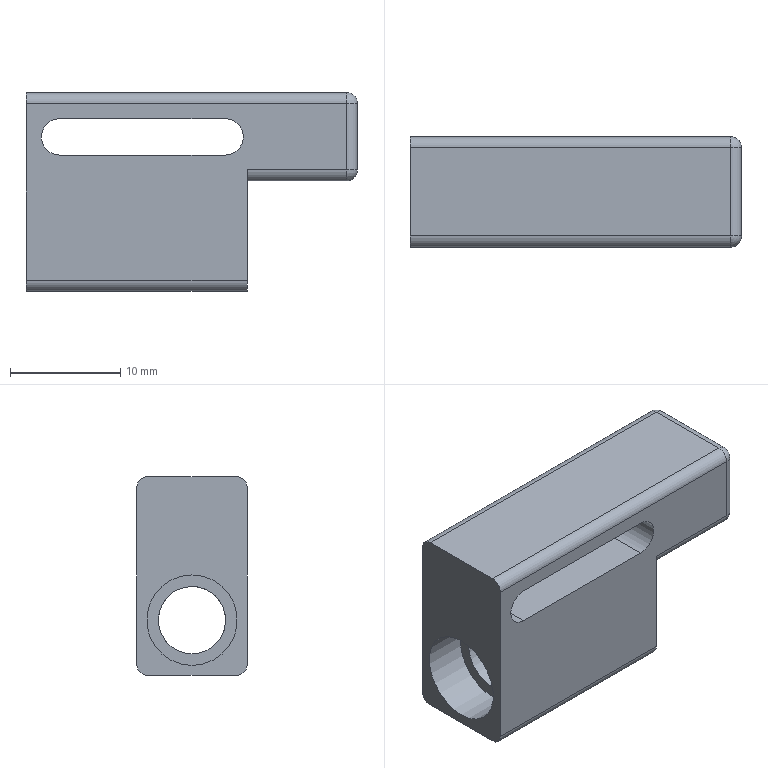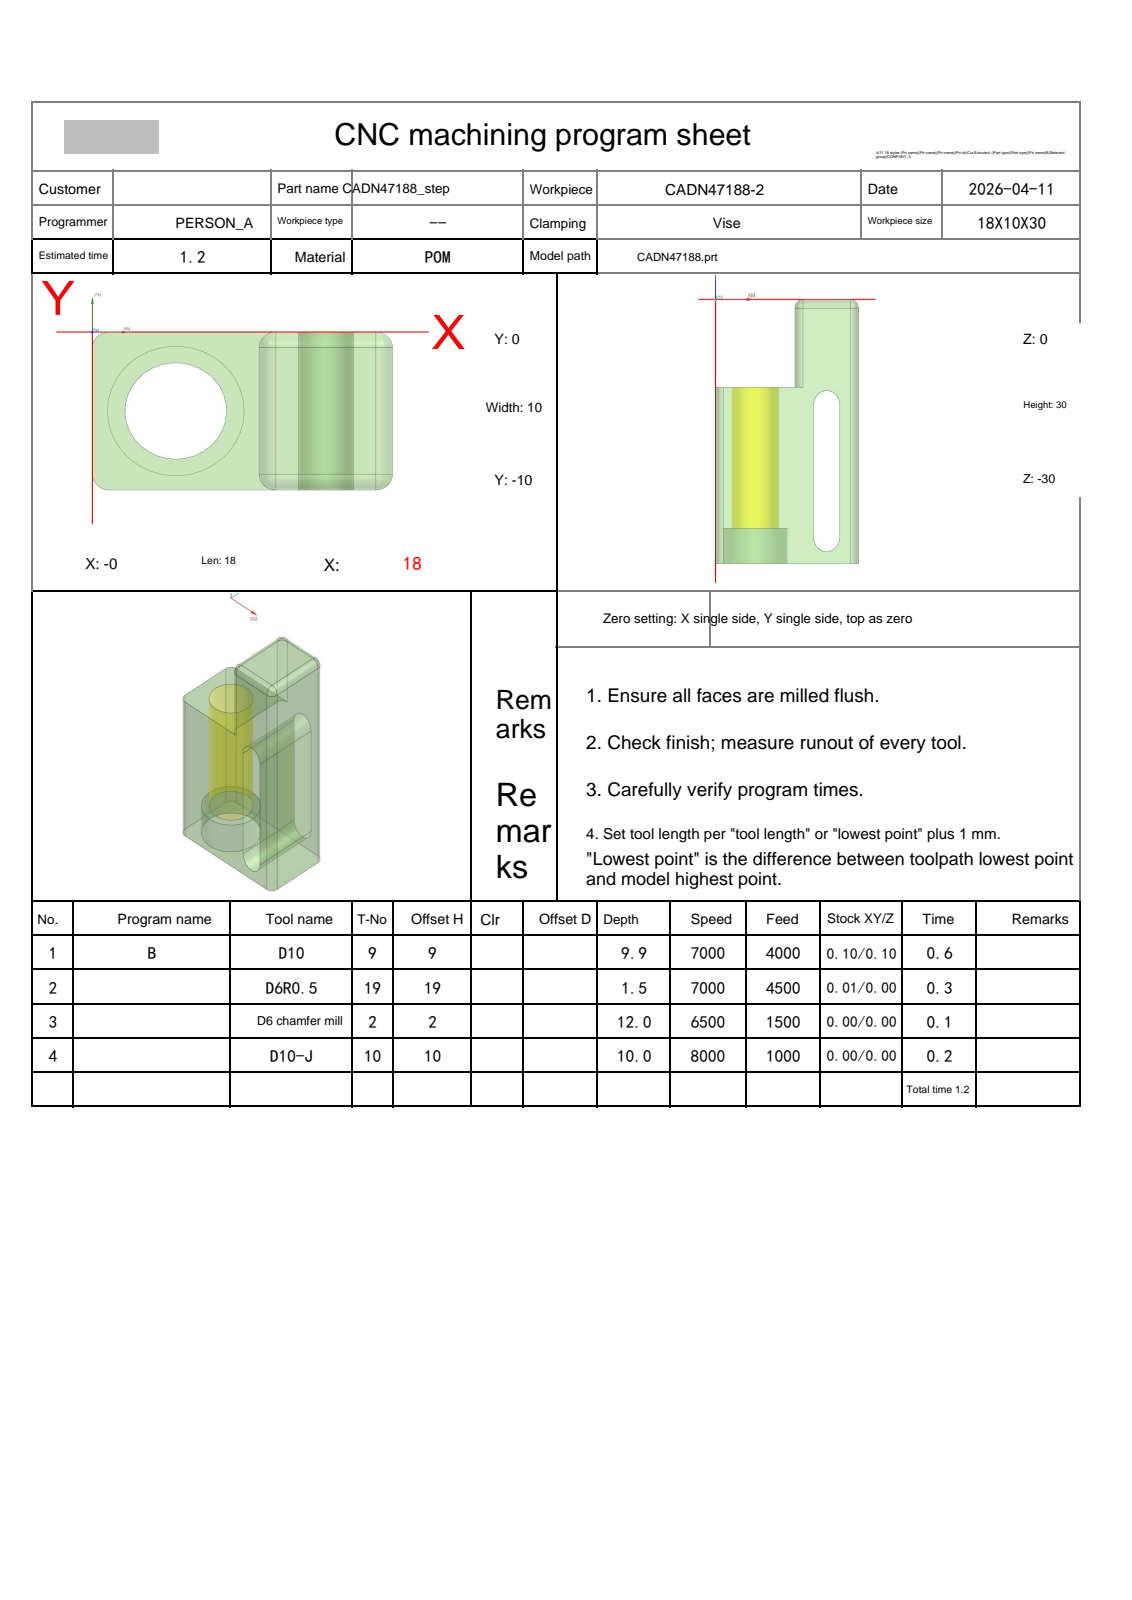NC program | NX | posted by the shop | part box 30 x 10 x 18 mm
Lines 1 to 456 of 3974:
%
O0001
(Machine time: 1.91 MIN)
(===Total Tool:4===)
(T9=D10     D=10.  R=0.   D-  H09 Z=-9.9  )
(T19=D6R0.5 D=6.   R=0.5  D-  H19 Z=-1.5  )
(T2=D6 chamfer mill   D=6.   R=0.   D-  H02 Z=-12.  )
(T10=D10-J  D=10.  R=0.   D10 H10 Z=-10.  )
G80 G90 G17 G49 G40
G91 G28 Z0
M01
N1 T09 M06
(D10  D=10. R=0. H=09 ce=0.10 di=0.10)
G00 G90 G54 X35.064 Y-10.094 M03 S7000
G43 H09 Z20.
M08
Z6.011
G01 Z4.011 F3000.
X22.998
X-4.097
G02 X-5.096 Y-9.113 I0.0 J1.
G01 X-5.097 Y-9.
Y-4.903
G02 X-4.097 Y-3.903 I1. J0.0
G01 X23.097
X35.097
Z6.011
G00 X35.064 Y-10.094
Z5.522
G01 Z3.522
X22.998
X-4.097
G02 X-5.096 Y-9.113 I0.0 J1.
G01 X-5.097 Y-9.
Y-4.903
G02 X-4.097 Y-3.903 I1. J0.0
G01 X23.097
X35.097
Z5.522
G00 X35.064 Y-10.094
Z5.033
G01 Z3.033
X22.998
X-4.097
G02 X-5.096 Y-9.113 I0.0 J1.
G01 X-5.097 Y-9.
Y-4.903
G02 X-4.097 Y-3.903 I1. J0.0
G01 X23.097
X35.097
Z5.033
G00 X35.064 Y-10.094
Z4.544
G01 Z2.544
X22.998
X-4.097
G02 X-5.096 Y-9.113 I0.0 J1.
G01 X-5.097 Y-9.
Y-4.903
G02 X-4.097 Y-3.903 I1. J0.0
G01 X23.097
X35.097
Z4.544
G00 X35.064 Y-10.094
Z4.056
G01 Z2.056
X22.998
X-4.097
G02 X-5.096 Y-9.113 I0.0 J1.
G01 X-5.097 Y-9.
Y-4.903
G02 X-4.097 Y-3.903 I1. J0.0
G01 X23.097
X35.097
Z4.056
G00 X35.064 Y-10.094
Z3.567
G01 Z1.567
X22.998
X-4.097
G02 X-5.096 Y-9.113 I0.0 J1.
G01 X-5.097 Y-9.
Y-4.903
G02 X-4.097 Y-3.903 I1. J0.0
G01 X23.097
X35.097
Z3.567
G00 X35.064 Y-10.094
Z3.078
G01 Z1.078
X22.998
X-4.097
G02 X-5.096 Y-9.113 I0.0 J1.
G01 X-5.097 Y-9.
Y-4.903
G02 X-4.097 Y-3.903 I1. J0.0
G01 X23.097
X35.097
Z3.078
G00 X35.064 Y-10.094
Z2.589
G01 Z.589
X22.998
X-4.097
G02 X-5.096 Y-9.113 I0.0 J1.
G01 X-5.097 Y-9.
Y-4.903
G02 X-4.097 Y-3.903 I1. J0.0
G01 X23.097
X35.097
Z2.589
G00 X35.064 Y-10.094
Z2.1
G01 Z.1
X22.998
X-4.097
G02 X-5.096 Y-9.113 I0.0 J1.
G01 X-5.097 Y-9.
Y-4.903
G02 X-4.097 Y-3.903 I1. J0.0
G01 X23.097
X35.097
Z2.1
G00 Z20.
G00 G90 X.033 Y7.948 M03 S7000
Z14.8
Z.918
G01 Z-.582 F4000.
X-1.508 Y4.341
G03 X-2.6 Y-1. I12.507 J-5.341
G01 Y-9.
G03 X-1.669 Y-13.946 I13.6 J0.0
X-1.092 Y-14.516 I.931 J.364
X1. Y-14.9 I2.092 J5.516
G01 X8.96 Y-16.839
G03 X9.197 Y-16.867 I.237 J.972
X10.197 Y-15.867 I0.0 J1.
X9.451 Y-14.9 I-1. J0.0
G02 X4.9 Y-9. I1.549 J5.9
G01 Y-1.
G02 X9.451 Y4.9 I6.1 J0.0
G01 X12.352 Y5.662
Y8.009
Z.918
G00 X.033 Y7.948
Z.335
G01 Z-1.165
X-1.508 Y4.341
G03 X-2.6 Y-1. I12.507 J-5.341
G01 Y-9.
G03 X-1.669 Y-13.946 I13.6 J0.0
X-1.092 Y-14.516 I.931 J.364
X1. Y-14.9 I2.092 J5.516
G01 X8.96 Y-16.839
G03 X9.197 Y-16.867 I.237 J.972
X10.197 Y-15.867 I0.0 J1.
X9.451 Y-14.9 I-1. J0.0
G02 X4.9 Y-9. I1.549 J5.9
G01 Y-1.
G02 X9.451 Y4.9 I6.1 J0.0
G01 X12.352 Y5.662
Y8.1
Z.335
G00 X.033 Y7.948
Z-.247
G01 Z-1.747
X-1.508 Y4.341
G03 X-2.6 Y-1. I12.507 J-5.341
G01 Y-9.
G03 X-1.669 Y-13.946 I13.6 J0.0
X-1.092 Y-14.516 I.931 J.364
X1. Y-14.9 I2.092 J5.516
G01 X8.96 Y-16.839
G03 X9.197 Y-16.867 I.237 J.972
X10.197 Y-15.867 I0.0 J1.
X9.451 Y-14.9 I-1. J0.0
G02 X4.9 Y-9. I1.549 J5.9
G01 Y-1.
G02 X9.451 Y4.9 I6.1 J0.0
G01 X12.352 Y5.662
Y8.1
Z-.247
G00 X.033 Y7.948
Z-.829
G01 Z-2.329
X-1.508 Y4.341
G03 X-2.6 Y-1. I12.507 J-5.341
G01 Y-9.
G03 X-1.669 Y-13.946 I13.6 J0.0
X-1.092 Y-14.516 I.931 J.364
X1. Y-14.9 I2.092 J5.516
G01 X8.96 Y-16.839
G03 X9.197 Y-16.867 I.237 J.972
X10.197 Y-15.867 I0.0 J1.
X9.451 Y-14.9 I-1. J0.0
G02 X4.9 Y-9. I1.549 J5.9
G01 Y-1.
G02 X9.451 Y4.9 I6.1 J0.0
G01 X12.352 Y5.662
Y8.1
Z-.829
G00 X.033 Y7.948
Z-1.412
G01 Z-2.912
X-1.508 Y4.341
G03 X-2.6 Y-1. I12.507 J-5.341
G01 Y-9.
G03 X-1.669 Y-13.946 I13.6 J0.0
X-1.092 Y-14.516 I.931 J.364
X1. Y-14.9 I2.092 J5.516
G01 X8.96 Y-16.839
G03 X9.197 Y-16.867 I.237 J.972
X10.197 Y-15.867 I0.0 J1.
X9.451 Y-14.9 I-1. J0.0
G02 X4.9 Y-9. I1.549 J5.9
G01 Y-1.
G02 X9.451 Y4.9 I6.1 J0.0
G01 X12.352 Y5.662
Y8.1
Z-1.412
G00 X.033 Y7.948
Z-1.994
G01 Z-3.494
X-1.508 Y4.341
G03 X-2.6 Y-1. I12.507 J-5.341
G01 Y-9.
G03 X-1.669 Y-13.946 I13.6 J0.0
X-1.092 Y-14.516 I.931 J.364
X1. Y-14.9 I2.092 J5.516
G01 X8.96 Y-16.839
G03 X9.197 Y-16.867 I.237 J.972
X10.197 Y-15.867 I0.0 J1.
X9.451 Y-14.9 I-1. J0.0
G02 X4.9 Y-9. I1.549 J5.9
G01 Y-1.
G02 X9.451 Y4.9 I6.1 J0.0
G01 X12.352 Y5.662
Y8.1
Z-1.994
G00 X.033 Y7.948
Z-2.576
G01 Z-4.076
X-1.508 Y4.341
G03 X-2.6 Y-1. I12.507 J-5.341
G01 Y-9.
G03 X-1.669 Y-13.946 I13.6 J0.0
X-1.092 Y-14.516 I.931 J.364
X1. Y-14.9 I2.092 J5.516
G01 X8.96 Y-16.839
G03 X9.197 Y-16.867 I.237 J.972
X10.197 Y-15.867 I0.0 J1.
X9.451 Y-14.9 I-1. J0.0
G02 X4.9 Y-9. I1.549 J5.9
G01 Y-1.
G02 X9.451 Y4.9 I6.1 J0.0
G01 X12.352 Y5.662
Y8.1
Z-2.576
G00 X.033 Y7.948
Z-3.159
G01 Z-4.659
X-1.508 Y4.341
G03 X-2.6 Y-1. I12.507 J-5.341
G01 Y-9.
G03 X-1.669 Y-13.946 I13.6 J0.0
X-1.092 Y-14.516 I.931 J.364
X1. Y-14.9 I2.092 J5.516
G01 X8.96 Y-16.839
G03 X9.197 Y-16.867 I.237 J.972
X10.197 Y-15.867 I0.0 J1.
X9.451 Y-14.9 I-1. J0.0
G02 X4.9 Y-9. I1.549 J5.9
G01 Y-1.
G02 X9.451 Y4.9 I6.1 J0.0
G01 X12.352 Y5.662
Y8.1
Z-3.159
G00 X.033 Y7.948
Z-3.741
G01 Z-5.241
X-1.508 Y4.341
G03 X-2.6 Y-1. I12.507 J-5.341
G01 Y-9.
G03 X-1.669 Y-13.946 I13.6 J0.0
X-1.092 Y-14.516 I.931 J.364
X1. Y-14.9 I2.092 J5.516
G01 X8.96 Y-16.839
G03 X9.197 Y-16.867 I.237 J.972
X10.197 Y-15.867 I0.0 J1.
X9.451 Y-14.9 I-1. J0.0
G02 X4.9 Y-9. I1.549 J5.9
G01 Y-1.
G02 X9.451 Y4.9 I6.1 J0.0
G01 X12.352 Y5.662
Y8.1
Z-3.741
G00 X.033 Y7.948
Z-4.324
G01 Z-5.824
X-1.508 Y4.341
G03 X-2.6 Y-1. I12.507 J-5.341
G01 Y-9.
G03 X-1.669 Y-13.946 I13.6 J0.0
X-1.092 Y-14.516 I.931 J.364
X1. Y-14.9 I2.092 J5.516
G01 X8.96 Y-16.839
G03 X9.197 Y-16.867 I.237 J.972
X10.197 Y-15.867 I0.0 J1.
X9.451 Y-14.9 I-1. J0.0
G02 X4.9 Y-9. I1.549 J5.9
G01 Y-1.
G02 X9.451 Y4.9 I6.1 J0.0
G01 X12.352 Y5.662
Y8.1
Z-4.324
G00 X.033 Y7.948
Z-4.906
G01 Z-6.406
X-1.508 Y4.341
G03 X-2.6 Y-1. I12.507 J-5.341
G01 Y-9.
G03 X-1.669 Y-13.946 I13.6 J0.0
X-1.092 Y-14.516 I.931 J.364
X1. Y-14.9 I2.092 J5.516
G01 X8.96 Y-16.839
G03 X9.197 Y-16.867 I.237 J.972
X10.197 Y-15.867 I0.0 J1.
X9.451 Y-14.9 I-1. J0.0
G02 X4.9 Y-9. I1.549 J5.9
G01 Y-1.
G02 X9.451 Y4.9 I6.1 J0.0
G01 X12.352 Y5.662
Y8.1
Z-4.906
G00 X.033 Y7.948
Z-5.488
G01 Z-6.988
X-1.508 Y4.341
G03 X-2.6 Y-1. I12.507 J-5.341
G01 Y-9.
G03 X-1.669 Y-13.946 I13.6 J0.0
X-1.092 Y-14.516 I.931 J.364
X1. Y-14.9 I2.092 J5.516
G01 X8.96 Y-16.839
G03 X9.197 Y-16.867 I.237 J.972
X10.197 Y-15.867 I0.0 J1.
X9.451 Y-14.9 I-1. J0.0
G02 X4.9 Y-9. I1.549 J5.9
G01 Y-1.
G02 X9.451 Y4.9 I6.1 J0.0
G01 X12.352 Y5.662
Y8.1
Z-5.488
G00 X.033 Y7.948
Z-6.071
G01 Z-7.571
X-1.508 Y4.341
G03 X-2.6 Y-1. I12.507 J-5.341
G01 Y-9.
G03 X-1.669 Y-13.946 I13.6 J0.0
X-1.092 Y-14.516 I.931 J.364
X1. Y-14.9 I2.092 J5.516
G01 X8.96 Y-16.839
G03 X9.197 Y-16.867 I.237 J.972
X10.197 Y-15.867 I0.0 J1.
X9.451 Y-14.9 I-1. J0.0
G02 X4.9 Y-9. I1.549 J5.9
G01 Y-1.
G02 X9.451 Y4.9 I6.1 J0.0
G01 X12.352 Y5.662
Y8.1
Z-6.071
G00 X.033 Y7.948
Z-6.653
G01 Z-8.153
X-1.508 Y4.341
G03 X-2.6 Y-1. I12.507 J-5.341
G01 Y-9.
G03 X-1.669 Y-13.946 I13.6 J0.0
X-1.092 Y-14.516 I.931 J.364
X1. Y-14.9 I2.092 J5.516
G01 X8.96 Y-16.839
G03 X9.197 Y-16.867 I.237 J.972
X10.197 Y-15.867 I0.0 J1.
X9.451 Y-14.9 I-1. J0.0
G02 X4.9 Y-9. I1.549 J5.9
G01 Y-1.
G02 X9.451 Y4.9 I6.1 J0.0
G01 X12.352 Y5.662
Y8.1
Z-6.653
G00 X.033 Y7.948
Z-7.235
G01 Z-8.735
X-1.508 Y4.341
G03 X-2.6 Y-1. I12.507 J-5.341
G01 Y-9.
G03 X-1.669 Y-13.946 I13.6 J0.0
X-1.092 Y-14.516 I.931 J.364
X1. Y-14.9 I2.092 J5.516
G01 X8.96 Y-16.839
G03 X9.197 Y-16.867 I.237 J.972
X10.197 Y-15.867 I0.0 J1.
X9.451 Y-14.9 I-1. J0.0
G02 X4.9 Y-9. I1.549 J5.9
G01 Y-1.
G02 X9.451 Y4.9 I6.1 J0.0
G01 X12.352 Y5.662
Y8.1
Z-7.235
G00 X.033 Y7.948
Z-7.818
G01 Z-9.318
X-1.508 Y4.341
G03 X-2.6 Y-1. I12.507 J-5.341
G01 Y-9.
G03 X-1.669 Y-13.946 I13.6 J0.0
X-1.092 Y-14.516 I.931 J.364
X1. Y-14.9 I2.092 J5.516
G01 X8.96 Y-16.839
G03 X9.197 Y-16.867 I.237 J.972
X10.197 Y-15.867 I0.0 J1.
X9.451 Y-14.9 I-1. J0.0
G02 X4.9 Y-9. I1.549 J5.9
G01 Y-1.
G02 X9.451 Y4.9 I6.1 J0.0
G01 X12.352 Y5.662
Y8.1
Z-7.818
G00 X.033 Y7.948
Z-8.4
G01 Z-9.9
X-1.508 Y4.341
G03 X-2.6 Y-1. I12.507 J-5.341
G01 Y-9.
G03 X-1.669 Y-13.946 I13.6 J0.0
X-1.092 Y-14.516 I.931 J.364
X1. Y-14.9 I2.092 J5.516
G01 X8.96 Y-16.839
G03 X9.197 Y-16.867 I.237 J.972
X10.197 Y-15.867 I0.0 J1.
X9.451 Y-14.9 I-1. J0.0
G02 X4.9 Y-9. I1.549 J5.9
G01 Y-1.
G02 X9.451 Y4.9 I6.1 J0.0
G01 X12.352 Y5.662
Y8.1
Z-8.4
G00 Z14.8
G91 G28 Z0.0
M05
M09
G91 G28 Z0.0
M01